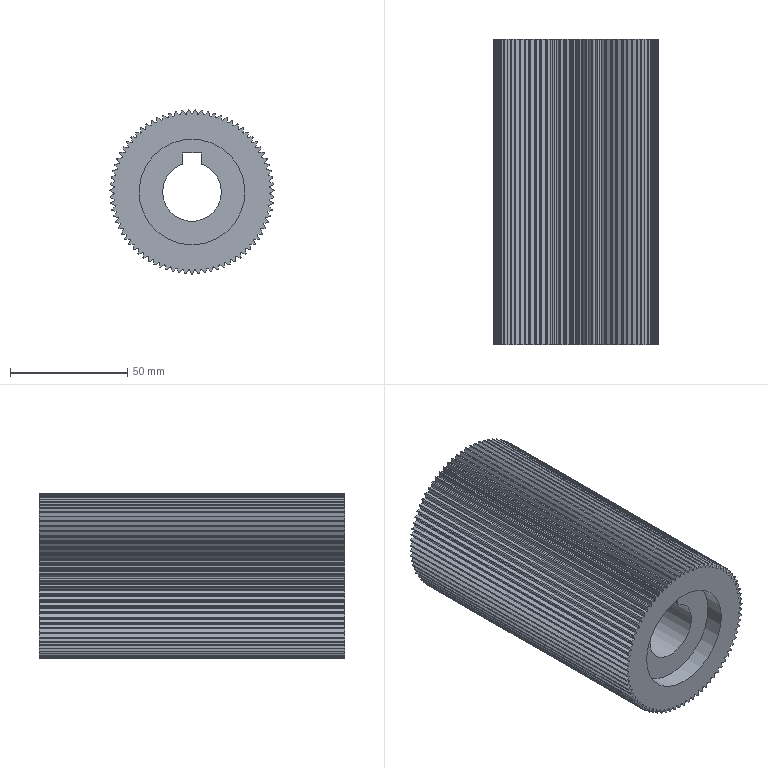Part | STEP file | YBQDJ-YB-15 | 1 solid | 326 faces | box 69.832 x 130 x 69.818 mm | volume 396551 mm3 | plane 164 | cylinder 162 | commonest cylinder face diameters 0.6 x158 0.8 x2 25 x1 45 x1